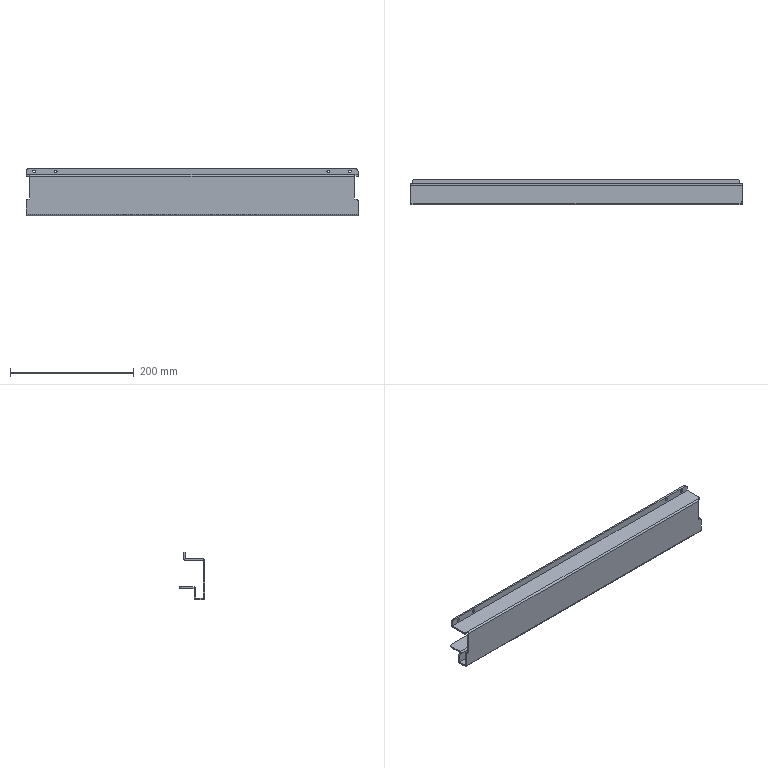Part | NX | features solid 2 | 1 solid | 97 faces | box 537.64 x 41.5 x 76.5 mm | volume 215467 mm3 | plane 56 | cylinder 41 | commonest cylinder face diameters 4.5 x20 5 x7 6 x6 5.3 x4 10 x4